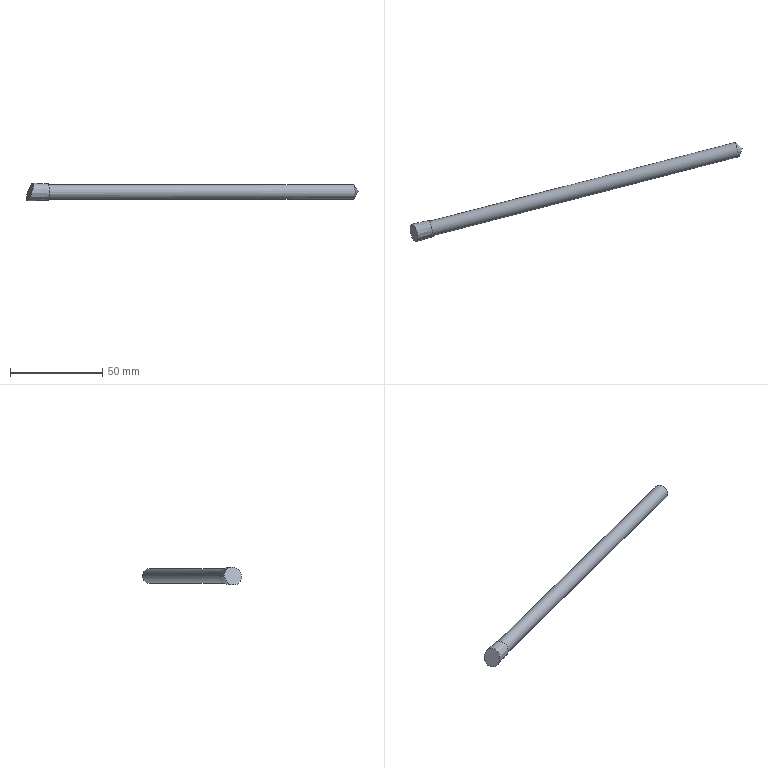Part | STEP file | 车灯-后视镜_id474_x_t | 1 solid | 5 faces | box 179.972 x 53.773 x 9.672 mm | volume 9329 mm3 | plane 2 | cone 2 | cylinder 1 | commonest cylinder face diameters 8 x1
STEP:
#1=CARTESIAN_POINT('',(-183.796,50.149,50.714));
#2=VERTEX_POINT('',#1);
#3=CARTESIAN_POINT('',(-182.798,46.275,50.714));
#4=DIRECTION('',(-0.9683,-0.2497,0.));
#5=DIRECTION('',(-0.2497,0.9683,0.));
#6=AXIS2_PLACEMENT_3D('',#3,#4,#5);
#7=CIRCLE('',#6,4.);
#8=EDGE_CURVE('',#2,#2,#7,.T.);
#9=ORIENTED_EDGE('',*,*,#8,.T.);
#10=EDGE_LOOP('',(#9));
#11=FACE_BOUND('',#10,.T.);
#12=CARTESIAN_POINT('',(-182.798,46.275,46.179));
#13=VERTEX_POINT('',#12);
#14=CARTESIAN_POINT('',(-182.798,46.275,50.714));
#15=DIRECTION('',(0.9683,0.2497,0.));
#16=DIRECTION('',(0.,0.,-1.));
#17=AXIS2_PLACEMENT_3D('',#14,#15,#16);
#18=CIRCLE('',#17,4.535);
#19=EDGE_CURVE('',#13,#13,#18,.T.);
#20=ORIENTED_EDGE('',*,*,#19,.T.);
#21=EDGE_LOOP('',(#20));
#22=FACE_BOUND('',#21,.T.);
#23=CARTESIAN_POINT('',(-182.798,46.275,50.714));
#24=DIRECTION('',(0.9683,0.2497,0.));
#25=DIRECTION('',(0.,0.,1.));
#26=AXIS2_PLACEMENT_3D('',#23,#24,#25);
#27=PLANE('',#26);
#28=ADVANCED_FACE('',(#11,#22),#27,.T.);
#29=CARTESIAN_POINT('',(-194.112,43.358,45.825));
#30=VERTEX_POINT('',#29);
#31=CARTESIAN_POINT('',(-192.407,43.797,50.661));
#32=DIRECTION('',(-0.9099,-0.2346,0.342));
#33=DIRECTION('',(-0.3312,-0.0854,-0.9397));
#34=AXIS2_PLACEMENT_3D('',#31,#32,#33);
#35=ELLIPSE('',#34,5.147,4.836);
#36=EDGE_CURVE('',#30,#30,#35,.T.);
#37=ORIENTED_EDGE('',*,*,#36,.F.);
#38=EDGE_LOOP('',(#37));
#39=FACE_BOUND('',#38,.T.);
#40=ORIENTED_EDGE('',*,*,#19,.F.);
#41=EDGE_LOOP('',(#40));
#42=FACE_BOUND('',#41,.T.);
#43=CARTESIAN_POINT('',(-182.798,46.275,50.714));
#44=DIRECTION('',(-0.9683,-0.2497,0.));
#45=DIRECTION('',(0.,0.,-1.));
#46=AXIS2_PLACEMENT_3D('',#43,#44,#45);
#47=CONICAL_SURFACE('',#46,4.535,1.738);
#48=ADVANCED_FACE('',(#39,#42),#47,.T.);
#49=ORIENTED_EDGE('',*,*,#8,.F.);
#50=EDGE_LOOP('',(#49));
#51=FACE_BOUND('',#50,.T.);
#52=CARTESIAN_POINT('',(-17.137,88.994,46.714));
#53=VERTEX_POINT('',#52);
#54=CARTESIAN_POINT('',(-17.137,88.994,50.714));
#55=DIRECTION('',(0.9683,0.2497,0.));
#56=DIRECTION('',(0.,0.,-1.));
#57=AXIS2_PLACEMENT_3D('',#54,#55,#56);
#58=CIRCLE('',#57,4.);
#59=EDGE_CURVE('',#53,#53,#58,.T.);
#60=ORIENTED_EDGE('',*,*,#59,.F.);
#61=EDGE_LOOP('',(#60));
#62=FACE_BOUND('',#61,.T.);
#63=CARTESIAN_POINT('',(-138.177,57.782,50.714));
#64=DIRECTION('',(0.9683,0.2497,0.));
#65=DIRECTION('',(0.,0.,1.));
#66=AXIS2_PLACEMENT_3D('',#63,#64,#65);
#67=CYLINDRICAL_SURFACE('',#66,4.);
#68=ADVANCED_FACE('',(#51,#62),#67,.T.);
#69=ORIENTED_EDGE('',*,*,#59,.T.);
#70=EDGE_LOOP('',(#69));
#71=FACE_BOUND('',#70,.T.);
#72=CARTESIAN_POINT('',(-14.524,89.668,50.714));
#73=VERTEX_POINT('',#72);
#74=VERTEX_LOOP('',#73);
#75=FACE_BOUND('',#74,.T.);
#76=CARTESIAN_POINT('',(-14.524,89.668,50.714));
#77=DIRECTION('',(-0.9683,-0.2497,0.));
#78=DIRECTION('',(0.,0.,1.));
#79=AXIS2_PLACEMENT_3D('',#76,#77,#78);
#80=CONICAL_SURFACE('',#79,0.,56.);
#81=ADVANCED_FACE('',(#71,#75),#80,.T.);
#82=ORIENTED_EDGE('',*,*,#36,.T.);
#83=EDGE_LOOP('',(#82));
#84=FACE_OUTER_BOUND('',#83,.T.);
#85=CARTESIAN_POINT('',(-192.52,23.906,36.714));
#86=DIRECTION('',(-0.9099,-0.2346,0.342));
#87=DIRECTION('',(0.3518,0.,0.9361));
#88=AXIS2_PLACEMENT_3D('',#85,#86,#87);
#89=PLANE('',#88);
#90=ADVANCED_FACE('',(#84),#89,.T.);
#91=CLOSED_SHELL('',(#28,#48,#68,#81,#90));
#92=MANIFOLD_SOLID_BREP('',#91);
#93=(LENGTH_UNIT()NAMED_UNIT(*)SI_UNIT(.MILLI.,.METRE.));
#94=UNCERTAINTY_MEASURE_WITH_UNIT(LENGTH_MEASURE(0.00002),#93,'','');
#95=(NAMED_UNIT(*)PLANE_ANGLE_UNIT()SI_UNIT($,.RADIAN.));
#96=PLANE_ANGLE_MEASURE_WITH_UNIT(PLANE_ANGLE_MEASURE(0.01745),#95);
#97=DIMENSIONAL_EXPONENTS(0.,0.,0.,0.,0.,0.,0.);
#98=(CONVERSION_BASED_UNIT('DEGREE',#96)NAMED_UNIT(#97)PLANE_ANGLE_UNIT());
#99=(NAMED_UNIT(*)SI_UNIT($,.STERADIAN.)SOLID_ANGLE_UNIT());
#100=(GEOMETRIC_REPRESENTATION_CONTEXT(3)GLOBAL_UNCERTAINTY_ASSIGNED_CONTEXT((#94))GLOBAL_UNIT_ASSIGNED_CONTEXT((#93,#98,#99))REPRESENTATION_CONTEXT('',''));
#101=ADVANCED_BREP_SHAPE_REPRESENTATION('',(#92),#100);